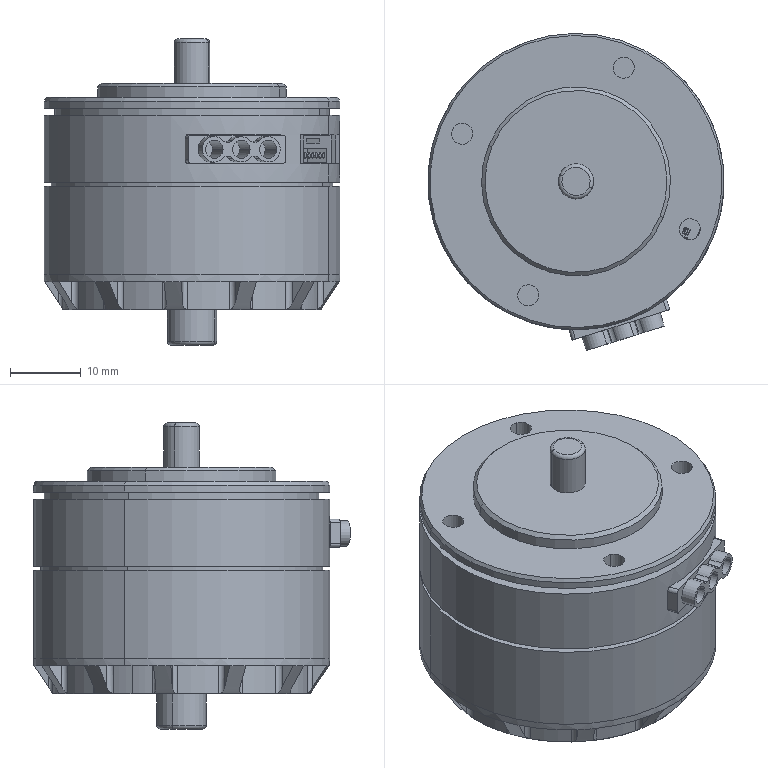Part | SolidWorks | features BaseBody 24, RefSurface 18 | 6 solids | 501 faces | box 42 x 44.967 x 43.4 mm | volume 38568 mm3 | plane 265 | cylinder 131 | spline 89 | cone 12 | torus 4 | commonest cylinder face diameters 1.4 x30 0.786 x14 36.56 x13 2 x8 2.5 x8 3 x8